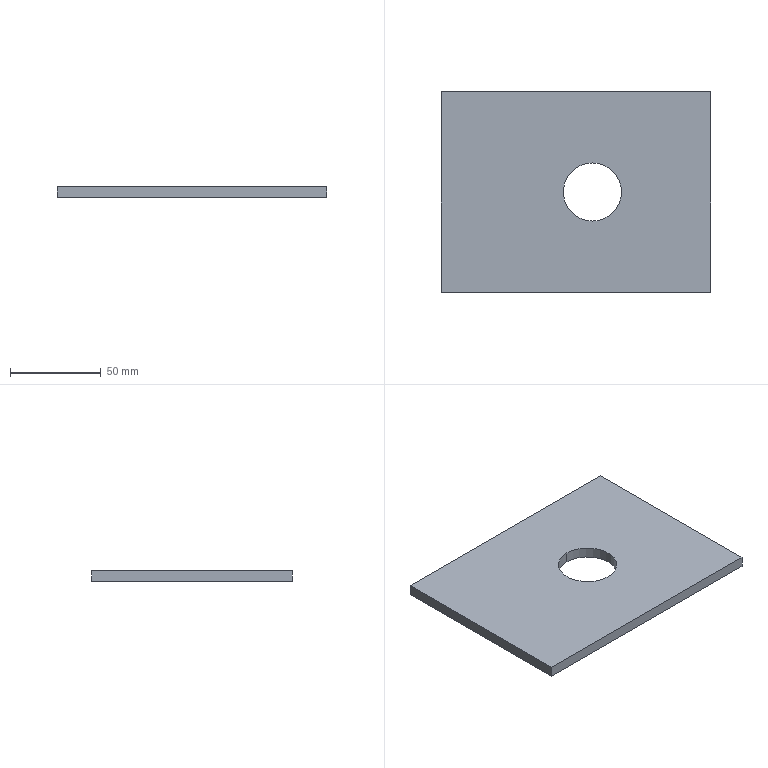Part | STEP file | 01-Pad plate | 1 solid | 8 faces | box 148 x 110 x 6 mm | volume 92855 mm3 | plane 6 | cylinder 2 | commonest cylinder face diameters 32 x2
STEP:
#1=CARTESIAN_POINT('',(0.,0.,0.));
#2=DIRECTION('',(0.,0.,1.));
#3=DIRECTION('',(1.,0.,0.));
#4=AXIS2_PLACEMENT_3D('',#1,#2,#3);
#5=CARTESIAN_POINT('',(83.,-39.,6.));
#6=VERTEX_POINT('',#5);
#7=CARTESIAN_POINT('',(83.,-39.,0.));
#8=VERTEX_POINT('',#7);
#9=CARTESIAN_POINT('',(83.,-39.,60.));
#10=DIRECTION('',(0.,0.,-1.));
#11=VECTOR('',#10,1.);
#12=LINE('',#9,#11);
#13=CARTESIAN_POINT('',(83.,-55.,60.));
#14=DIRECTION('',(0.,0.,-1.));
#15=DIRECTION('',(0.,1.,0.));
#16=AXIS2_PLACEMENT_3D('',#13,#14,#15);
#17=CYLINDRICAL_SURFACE('',#16,16.);
#18=CARTESIAN_POINT('',(6.283,0.));
#19=DIRECTION('',(0.,1.));
#20=VECTOR('',#19,1.);
#21=LINE('',#18,#20);
#22=(GEOMETRIC_REPRESENTATION_CONTEXT(2)PARAMETRIC_REPRESENTATION_CONTEXT()REPRESENTATION_CONTEXT('',''));
#23=DEFINITIONAL_REPRESENTATION('',(#21),#22);
#24=PCURVE('',#17,#23);
#25=CARTESIAN_POINT('',(83.,-55.,60.));
#26=DIRECTION('',(0.,0.,-1.));
#27=DIRECTION('',(0.,1.,0.));
#28=AXIS2_PLACEMENT_3D('',#25,#26,#27);
#29=CYLINDRICAL_SURFACE('',#28,16.);
#30=CARTESIAN_POINT('',(0.,0.));
#31=DIRECTION('',(0.,1.));
#32=VECTOR('',#31,1.);
#33=LINE('',#30,#32);
#34=(GEOMETRIC_REPRESENTATION_CONTEXT(2)PARAMETRIC_REPRESENTATION_CONTEXT()REPRESENTATION_CONTEXT('',''));
#35=DEFINITIONAL_REPRESENTATION('',(#33),#34);
#36=PCURVE('',#29,#35);
#37=SURFACE_CURVE('',#12,(#24,#36),.PCURVE_S1.);
#38=EDGE_CURVE('',#6,#8,#37,.T.);
#39=ORIENTED_EDGE('',*,*,#38,.T.);
#40=CARTESIAN_POINT('',(83.,-71.,0.));
#41=VERTEX_POINT('',#40);
#42=CARTESIAN_POINT('',(83.,-55.,0.));
#43=DIRECTION('',(0.,0.,-1.));
#44=DIRECTION('',(0.,1.,0.));
#45=AXIS2_PLACEMENT_3D('',#42,#43,#44);
#46=CIRCLE('',#45,16.);
#47=CARTESIAN_POINT('',(0.,60.));
#48=DIRECTION('',(1.,0.));
#49=VECTOR('',#48,1.);
#50=LINE('',#47,#49);
#51=(GEOMETRIC_REPRESENTATION_CONTEXT(2)PARAMETRIC_REPRESENTATION_CONTEXT()REPRESENTATION_CONTEXT('',''));
#52=DEFINITIONAL_REPRESENTATION('',(#50),#51);
#53=PCURVE('',#17,#52);
#54=CARTESIAN_POINT('',(0.,0.,0.));
#55=DIRECTION('',(0.,0.,1.));
#56=DIRECTION('',(1.,0.,0.));
#57=AXIS2_PLACEMENT_3D('',#54,#55,#56);
#58=PLANE('',#57);
#59=CARTESIAN_POINT('',(83.,-39.));
#60=CARTESIAN_POINT('',(110.713,-39.));
#61=CARTESIAN_POINT('',(96.856,-63.));
#62=CARTESIAN_POINT('',(83.,-87.));
#63=CARTESIAN_POINT('',(69.144,-63.));
#64=CARTESIAN_POINT('',(55.287,-39.));
#65=CARTESIAN_POINT('',(83.,-39.));
#66=(BOUNDED_CURVE()B_SPLINE_CURVE(2,(#59,#60,#61,#62,#63,#64,#65),.UNSPECIFIED.,.T.,.F.)B_SPLINE_CURVE_WITH_KNOTS((1,2,2,2,2,1),(-2.094,0.,2.094,4.189,6.283,8.378),.UNSPECIFIED.)CURVE()GEOMETRIC_REPRESENTATION_ITEM()RATIONAL_B_SPLINE_CURVE((1.,0.5,1.,0.5,1.,0.5,1.))REPRESENTATION_ITEM(''));
#67=(GEOMETRIC_REPRESENTATION_CONTEXT(2)PARAMETRIC_REPRESENTATION_CONTEXT()REPRESENTATION_CONTEXT('',''));
#68=DEFINITIONAL_REPRESENTATION('',(#66),#67);
#69=PCURVE('',#58,#68);
#70=SURFACE_CURVE('',#46,(#53,#69),.PCURVE_S1.);
#71=EDGE_CURVE('',#41,#8,#70,.T.);
#72=ORIENTED_EDGE('',*,*,#71,.F.);
#73=CARTESIAN_POINT('',(83.,-71.,6.));
#74=VERTEX_POINT('',#73);
#75=CARTESIAN_POINT('',(83.,-71.,60.));
#76=DIRECTION('',(0.,0.,-1.));
#77=VECTOR('',#76,1.);
#78=LINE('',#75,#77);
#79=CARTESIAN_POINT('',(3.142,0.));
#80=DIRECTION('',(0.,1.));
#81=VECTOR('',#80,1.);
#82=LINE('',#79,#81);
#83=(GEOMETRIC_REPRESENTATION_CONTEXT(2)PARAMETRIC_REPRESENTATION_CONTEXT()REPRESENTATION_CONTEXT('',''));
#84=DEFINITIONAL_REPRESENTATION('',(#82),#83);
#85=PCURVE('',#17,#84);
#86=CARTESIAN_POINT('',(3.142,0.));
#87=DIRECTION('',(0.,1.));
#88=VECTOR('',#87,1.);
#89=LINE('',#86,#88);
#90=(GEOMETRIC_REPRESENTATION_CONTEXT(2)PARAMETRIC_REPRESENTATION_CONTEXT()REPRESENTATION_CONTEXT('',''));
#91=DEFINITIONAL_REPRESENTATION('',(#89),#90);
#92=PCURVE('',#29,#91);
#93=SURFACE_CURVE('',#78,(#85,#92),.PCURVE_S1.);
#94=EDGE_CURVE('',#74,#41,#93,.T.);
#95=ORIENTED_EDGE('',*,*,#94,.F.);
#96=CARTESIAN_POINT('',(83.,-55.,6.));
#97=DIRECTION('',(0.,0.,1.));
#98=DIRECTION('',(0.,-1.,0.));
#99=AXIS2_PLACEMENT_3D('',#96,#97,#98);
#100=CIRCLE('',#99,16.);
#101=CARTESIAN_POINT('',(9.425,54.));
#102=DIRECTION('',(-1.,0.));
#103=VECTOR('',#102,1.);
#104=LINE('',#101,#103);
#105=(GEOMETRIC_REPRESENTATION_CONTEXT(2)PARAMETRIC_REPRESENTATION_CONTEXT()REPRESENTATION_CONTEXT('',''));
#106=DEFINITIONAL_REPRESENTATION('',(#104),#105);
#107=PCURVE('',#17,#106);
#108=CARTESIAN_POINT('',(0.,0.,6.));
#109=DIRECTION('',(0.,0.,1.));
#110=DIRECTION('',(1.,0.,0.));
#111=AXIS2_PLACEMENT_3D('',#108,#109,#110);
#112=PLANE('',#111);
#113=CARTESIAN_POINT('',(83.,-55.));
#114=DIRECTION('',(0.,-1.));
#115=AXIS2_PLACEMENT_2D('',#113,#114);
#116=CIRCLE('',#115,16.);
#117=(GEOMETRIC_REPRESENTATION_CONTEXT(2)PARAMETRIC_REPRESENTATION_CONTEXT()REPRESENTATION_CONTEXT('',''));
#118=DEFINITIONAL_REPRESENTATION('',(#116),#117);
#119=PCURVE('',#112,#118);
#120=SURFACE_CURVE('',#100,(#107,#119),.PCURVE_S1.);
#121=EDGE_CURVE('',#6,#74,#120,.T.);
#122=ORIENTED_EDGE('',*,*,#121,.F.);
#123=EDGE_LOOP('',(#39,#72,#95,#122));
#124=FACE_BOUND('',#123,.F.);
#125=ADVANCED_FACE('',(#124),#17,.F.);
#126=CARTESIAN_POINT('',(0.,0.,0.));
#127=VERTEX_POINT('',#126);
#128=CARTESIAN_POINT('',(0.,-110.,0.));
#129=VERTEX_POINT('',#128);
#130=CARTESIAN_POINT('',(0.,0.,0.));
#131=DIRECTION('',(0.,-1.,0.));
#132=VECTOR('',#131,1.);
#133=LINE('',#130,#132);
#134=CARTESIAN_POINT('',(0.,0.,6.));
#135=DIRECTION('',(1.,0.,0.));
#136=DIRECTION('',(0.,1.,0.));
#137=AXIS2_PLACEMENT_3D('',#134,#135,#136);
#138=PLANE('',#137);
#139=CARTESIAN_POINT('',(0.,-6.));
#140=DIRECTION('',(-1.,0.));
#141=VECTOR('',#140,1.);
#142=LINE('',#139,#141);
#143=(GEOMETRIC_REPRESENTATION_CONTEXT(2)PARAMETRIC_REPRESENTATION_CONTEXT()REPRESENTATION_CONTEXT('',''));
#144=DEFINITIONAL_REPRESENTATION('',(#142),#143);
#145=PCURVE('',#138,#144);
#146=CARTESIAN_POINT('',(0.,0.));
#147=DIRECTION('',(0.,-1.));
#148=VECTOR('',#147,1.);
#149=LINE('',#146,#148);
#150=(GEOMETRIC_REPRESENTATION_CONTEXT(2)PARAMETRIC_REPRESENTATION_CONTEXT()REPRESENTATION_CONTEXT('',''));
#151=DEFINITIONAL_REPRESENTATION('',(#149),#150);
#152=PCURVE('',#58,#151);
#153=SURFACE_CURVE('',#133,(#145,#152),.PCURVE_S1.);
#154=EDGE_CURVE('',#127,#129,#153,.T.);
#155=ORIENTED_EDGE('',*,*,#154,.T.);
#156=CARTESIAN_POINT('',(0.,-110.,6.));
#157=VERTEX_POINT('',#156);
#158=CARTESIAN_POINT('',(0.,-110.,6.));
#159=DIRECTION('',(0.,0.,-1.));
#160=VECTOR('',#159,1.);
#161=LINE('',#158,#160);
#162=CARTESIAN_POINT('',(-110.,0.));
#163=DIRECTION('',(0.,-1.));
#164=VECTOR('',#163,1.);
#165=LINE('',#162,#164);
#166=(GEOMETRIC_REPRESENTATION_CONTEXT(2)PARAMETRIC_REPRESENTATION_CONTEXT()REPRESENTATION_CONTEXT('',''));
#167=DEFINITIONAL_REPRESENTATION('',(#165),#166);
#168=PCURVE('',#138,#167);
#169=CARTESIAN_POINT('',(0.,-110.,6.));
#170=DIRECTION('',(0.,1.,0.));
#171=DIRECTION('',(0.,0.,1.));
#172=AXIS2_PLACEMENT_3D('',#169,#170,#171);
#173=PLANE('',#172);
#174=CARTESIAN_POINT('',(0.,0.));
#175=DIRECTION('',(-1.,0.));
#176=VECTOR('',#175,1.);
#177=LINE('',#174,#176);
#178=(GEOMETRIC_REPRESENTATION_CONTEXT(2)PARAMETRIC_REPRESENTATION_CONTEXT()REPRESENTATION_CONTEXT('',''));
#179=DEFINITIONAL_REPRESENTATION('',(#177),#178);
#180=PCURVE('',#173,#179);
#181=SURFACE_CURVE('',#161,(#168,#180),.PCURVE_S1.);
#182=EDGE_CURVE('',#157,#129,#181,.T.);
#183=ORIENTED_EDGE('',*,*,#182,.F.);
#184=CARTESIAN_POINT('',(0.,0.,6.));
#185=VERTEX_POINT('',#184);
#186=CARTESIAN_POINT('',(0.,0.,6.));
#187=DIRECTION('',(0.,-1.,0.));
#188=VECTOR('',#187,1.);
#189=LINE('',#186,#188);
#190=CARTESIAN_POINT('',(0.,0.));
#191=DIRECTION('',(-1.,0.));
#192=VECTOR('',#191,1.);
#193=LINE('',#190,#192);
#194=(GEOMETRIC_REPRESENTATION_CONTEXT(2)PARAMETRIC_REPRESENTATION_CONTEXT()REPRESENTATION_CONTEXT('',''));
#195=DEFINITIONAL_REPRESENTATION('',(#193),#194);
#196=PCURVE('',#138,#195);
#197=CARTESIAN_POINT('',(0.,0.));
#198=DIRECTION('',(0.,-1.));
#199=VECTOR('',#198,1.);
#200=LINE('',#197,#199);
#201=(GEOMETRIC_REPRESENTATION_CONTEXT(2)PARAMETRIC_REPRESENTATION_CONTEXT()REPRESENTATION_CONTEXT('',''));
#202=DEFINITIONAL_REPRESENTATION('',(#200),#201);
#203=PCURVE('',#112,#202);
#204=SURFACE_CURVE('',#189,(#196,#203),.PCURVE_S1.);
#205=EDGE_CURVE('',#185,#157,#204,.T.);
#206=ORIENTED_EDGE('',*,*,#205,.F.);
#207=CARTESIAN_POINT('',(0.,0.,6.));
#208=DIRECTION('',(0.,0.,-1.));
#209=VECTOR('',#208,1.);
#210=LINE('',#207,#209);
#211=CARTESIAN_POINT('',(0.,0.));
#212=DIRECTION('',(0.,-1.));
#213=VECTOR('',#212,1.);
#214=LINE('',#211,#213);
#215=(GEOMETRIC_REPRESENTATION_CONTEXT(2)PARAMETRIC_REPRESENTATION_CONTEXT()REPRESENTATION_CONTEXT('',''));
#216=DEFINITIONAL_REPRESENTATION('',(#214),#215);
#217=PCURVE('',#138,#216);
#218=CARTESIAN_POINT('',(0.,0.,6.));
#219=DIRECTION('',(0.,-1.,0.));
#220=DIRECTION('',(0.,0.,-1.));
#221=AXIS2_PLACEMENT_3D('',#218,#219,#220);
#222=PLANE('',#221);
#223=CARTESIAN_POINT('',(0.,0.));
#224=DIRECTION('',(1.,0.));
#225=VECTOR('',#224,1.);
#226=LINE('',#223,#225);
#227=(GEOMETRIC_REPRESENTATION_CONTEXT(2)PARAMETRIC_REPRESENTATION_CONTEXT()REPRESENTATION_CONTEXT('',''));
#228=DEFINITIONAL_REPRESENTATION('',(#226),#227);
#229=PCURVE('',#222,#228);
#230=SURFACE_CURVE('',#210,(#217,#229),.PCURVE_S1.);
#231=EDGE_CURVE('',#185,#127,#230,.T.);
#232=ORIENTED_EDGE('',*,*,#231,.T.);
#233=EDGE_LOOP('',(#155,#183,#206,#232));
#234=FACE_BOUND('',#233,.T.);
#235=ADVANCED_FACE('',(#234),#138,.F.);
#236=CARTESIAN_POINT('',(148.,-110.,0.));
#237=VERTEX_POINT('',#236);
#238=CARTESIAN_POINT('',(0.,-110.,0.));
#239=DIRECTION('',(1.,0.,0.));
#240=VECTOR('',#239,1.);
#241=LINE('',#238,#240);
#242=CARTESIAN_POINT('',(-6.,0.));
#243=DIRECTION('',(0.,1.));
#244=VECTOR('',#243,1.);
#245=LINE('',#242,#244);
#246=(GEOMETRIC_REPRESENTATION_CONTEXT(2)PARAMETRIC_REPRESENTATION_CONTEXT()REPRESENTATION_CONTEXT('',''));
#247=DEFINITIONAL_REPRESENTATION('',(#245),#246);
#248=PCURVE('',#173,#247);
#249=CARTESIAN_POINT('',(0.,-110.));
#250=DIRECTION('',(1.,0.));
#251=VECTOR('',#250,1.);
#252=LINE('',#249,#251);
#253=(GEOMETRIC_REPRESENTATION_CONTEXT(2)PARAMETRIC_REPRESENTATION_CONTEXT()REPRESENTATION_CONTEXT('',''));
#254=DEFINITIONAL_REPRESENTATION('',(#252),#253);
#255=PCURVE('',#58,#254);
#256=SURFACE_CURVE('',#241,(#248,#255),.PCURVE_S1.);
#257=EDGE_CURVE('',#129,#237,#256,.T.);
#258=ORIENTED_EDGE('',*,*,#257,.T.);
#259=CARTESIAN_POINT('',(148.,-110.,6.));
#260=VERTEX_POINT('',#259);
#261=CARTESIAN_POINT('',(148.,-110.,6.));
#262=DIRECTION('',(0.,0.,-1.));
#263=VECTOR('',#262,1.);
#264=LINE('',#261,#263);
#265=CARTESIAN_POINT('',(0.,148.));
#266=DIRECTION('',(-1.,0.));
#267=VECTOR('',#266,1.);
#268=LINE('',#265,#267);
#269=(GEOMETRIC_REPRESENTATION_CONTEXT(2)PARAMETRIC_REPRESENTATION_CONTEXT()REPRESENTATION_CONTEXT('',''));
#270=DEFINITIONAL_REPRESENTATION('',(#268),#269);
#271=PCURVE('',#173,#270);
#272=CARTESIAN_POINT('',(148.,0.,6.));
#273=DIRECTION('',(-1.,0.,0.));
#274=DIRECTION('',(0.,0.,1.));
#275=AXIS2_PLACEMENT_3D('',#272,#273,#274);
#276=PLANE('',#275);
#277=CARTESIAN_POINT('',(0.,-110.));
#278=DIRECTION('',(-1.,0.));
#279=VECTOR('',#278,1.);
#280=LINE('',#277,#279);
#281=(GEOMETRIC_REPRESENTATION_CONTEXT(2)PARAMETRIC_REPRESENTATION_CONTEXT()REPRESENTATION_CONTEXT('',''));
#282=DEFINITIONAL_REPRESENTATION('',(#280),#281);
#283=PCURVE('',#276,#282);
#284=SURFACE_CURVE('',#264,(#271,#283),.PCURVE_S1.);
#285=EDGE_CURVE('',#260,#237,#284,.T.);
#286=ORIENTED_EDGE('',*,*,#285,.F.);
#287=CARTESIAN_POINT('',(0.,-110.,6.));
#288=DIRECTION('',(1.,0.,0.));
#289=VECTOR('',#288,1.);
#290=LINE('',#287,#289);
#291=CARTESIAN_POINT('',(0.,0.));
#292=DIRECTION('',(0.,1.));
#293=VECTOR('',#292,1.);
#294=LINE('',#291,#293);
#295=(GEOMETRIC_REPRESENTATION_CONTEXT(2)PARAMETRIC_REPRESENTATION_CONTEXT()REPRESENTATION_CONTEXT('',''));
#296=DEFINITIONAL_REPRESENTATION('',(#294),#295);
#297=PCURVE('',#173,#296);
#298=CARTESIAN_POINT('',(0.,-110.));
#299=DIRECTION('',(1.,0.));
#300=VECTOR('',#299,1.);
#301=LINE('',#298,#300);
#302=(GEOMETRIC_REPRESENTATION_CONTEXT(2)PARAMETRIC_REPRESENTATION_CONTEXT()REPRESENTATION_CONTEXT('',''));
#303=DEFINITIONAL_REPRESENTATION('',(#301),#302);
#304=PCURVE('',#112,#303);
#305=SURFACE_CURVE('',#290,(#297,#304),.PCURVE_S1.);
#306=EDGE_CURVE('',#157,#260,#305,.T.);
#307=ORIENTED_EDGE('',*,*,#306,.F.);
#308=ORIENTED_EDGE('',*,*,#182,.T.);
#309=EDGE_LOOP('',(#258,#286,#307,#308));
#310=FACE_BOUND('',#309,.T.);
#311=ADVANCED_FACE('',(#310),#173,.F.);
#312=CARTESIAN_POINT('',(148.,0.,0.));
#313=VERTEX_POINT('',#312);
#314=CARTESIAN_POINT('',(148.,0.,0.));
#315=DIRECTION('',(0.,1.,0.));
#316=VECTOR('',#315,1.);
#317=LINE('',#314,#316);
#318=CARTESIAN_POINT('',(-6.,0.));
#319=DIRECTION('',(0.,1.));
#320=VECTOR('',#319,1.);
#321=LINE('',#318,#320);
#322=(GEOMETRIC_REPRESENTATION_CONTEXT(2)PARAMETRIC_REPRESENTATION_CONTEXT()REPRESENTATION_CONTEXT('',''));
#323=DEFINITIONAL_REPRESENTATION('',(#321),#322);
#324=PCURVE('',#276,#323);
#325=CARTESIAN_POINT('',(148.,0.));
#326=DIRECTION('',(0.,1.));
#327=VECTOR('',#326,1.);
#328=LINE('',#325,#327);
#329=(GEOMETRIC_REPRESENTATION_CONTEXT(2)PARAMETRIC_REPRESENTATION_CONTEXT()REPRESENTATION_CONTEXT('',''));
#330=DEFINITIONAL_REPRESENTATION('',(#328),#329);
#331=PCURVE('',#58,#330);
#332=SURFACE_CURVE('',#317,(#324,#331),.PCURVE_S1.);
#333=EDGE_CURVE('',#237,#313,#332,.T.);
#334=ORIENTED_EDGE('',*,*,#333,.T.);
#335=CARTESIAN_POINT('',(148.,0.,6.));
#336=VERTEX_POINT('',#335);
#337=CARTESIAN_POINT('',(148.,0.,6.));
#338=DIRECTION('',(0.,0.,-1.));
#339=VECTOR('',#338,1.);
#340=LINE('',#337,#339);
#341=CARTESIAN_POINT('',(0.,0.));
#342=DIRECTION('',(-1.,0.));
#343=VECTOR('',#342,1.);
#344=LINE('',#341,#343);
#345=(GEOMETRIC_REPRESENTATION_CONTEXT(2)PARAMETRIC_REPRESENTATION_CONTEXT()REPRESENTATION_CONTEXT('',''));
#346=DEFINITIONAL_REPRESENTATION('',(#344),#345);
#347=PCURVE('',#276,#346);
#348=CARTESIAN_POINT('',(0.,148.));
#349=DIRECTION('',(1.,0.));
#350=VECTOR('',#349,1.);
#351=LINE('',#348,#350);
#352=(GEOMETRIC_REPRESENTATION_CONTEXT(2)PARAMETRIC_REPRESENTATION_CONTEXT()REPRESENTATION_CONTEXT('',''));
#353=DEFINITIONAL_REPRESENTATION('',(#351),#352);
#354=PCURVE('',#222,#353);
#355=SURFACE_CURVE('',#340,(#347,#354),.PCURVE_S1.);
#356=EDGE_CURVE('',#336,#313,#355,.T.);
#357=ORIENTED_EDGE('',*,*,#356,.F.);
#358=CARTESIAN_POINT('',(148.,0.,6.));
#359=DIRECTION('',(0.,1.,0.));
#360=VECTOR('',#359,1.);
#361=LINE('',#358,#360);
#362=CARTESIAN_POINT('',(0.,0.));
#363=DIRECTION('',(0.,1.));
#364=VECTOR('',#363,1.);
#365=LINE('',#362,#364);
#366=(GEOMETRIC_REPRESENTATION_CONTEXT(2)PARAMETRIC_REPRESENTATION_CONTEXT()REPRESENTATION_CONTEXT('',''));
#367=DEFINITIONAL_REPRESENTATION('',(#365),#366);
#368=PCURVE('',#276,#367);
#369=CARTESIAN_POINT('',(148.,0.));
#370=DIRECTION('',(0.,1.));
#371=VECTOR('',#370,1.);
#372=LINE('',#369,#371);
#373=(GEOMETRIC_REPRESENTATION_CONTEXT(2)PARAMETRIC_REPRESENTATION_CONTEXT()REPRESENTATION_CONTEXT('',''));
#374=DEFINITIONAL_REPRESENTATION('',(#372),#373);
#375=PCURVE('',#112,#374);
#376=SURFACE_CURVE('',#361,(#368,#375),.PCURVE_S1.);
#377=EDGE_CURVE('',#260,#336,#376,.T.);
#378=ORIENTED_EDGE('',*,*,#377,.F.);
#379=ORIENTED_EDGE('',*,*,#285,.T.);
#380=EDGE_LOOP('',(#334,#357,#378,#379));
#381=FACE_BOUND('',#380,.T.);
#382=ADVANCED_FACE('',(#381),#276,.F.);
#383=CARTESIAN_POINT('',(0.,0.,0.));
#384=DIRECTION('',(-1.,0.,0.));
#385=VECTOR('',#384,1.);
#386=LINE('',#383,#385);
#387=CARTESIAN_POINT('',(6.,0.));
#388=DIRECTION('',(0.,-1.));
#389=VECTOR('',#388,1.);
#390=LINE('',#387,#389);
#391=(GEOMETRIC_REPRESENTATION_CONTEXT(2)PARAMETRIC_REPRESENTATION_CONTEXT()REPRESENTATION_CONTEXT('',''));
#392=DEFINITIONAL_REPRESENTATION('',(#390),#391);
#393=PCURVE('',#222,#392);
#394=CARTESIAN_POINT('',(0.,0.));
#395=DIRECTION('',(-1.,0.));
#396=VECTOR('',#395,1.);
#397=LINE('',#394,#396);
#398=(GEOMETRIC_REPRESENTATION_CONTEXT(2)PARAMETRIC_REPRESENTATION_CONTEXT()REPRESENTATION_CONTEXT('',''));
#399=DEFINITIONAL_REPRESENTATION('',(#397),#398);
#400=PCURVE('',#58,#399);
#401=SURFACE_CURVE('',#386,(#393,#400),.PCURVE_S1.);
#402=EDGE_CURVE('',#313,#127,#401,.T.);
#403=ORIENTED_EDGE('',*,*,#402,.T.);
#404=ORIENTED_EDGE('',*,*,#231,.F.);
#405=CARTESIAN_POINT('',(0.,0.,6.));
#406=DIRECTION('',(-1.,0.,0.));
#407=VECTOR('',#406,1.);
#408=LINE('',#405,#407);
#409=CARTESIAN_POINT('',(0.,0.));
#410=DIRECTION('',(0.,-1.));
#411=VECTOR('',#410,1.);
#412=LINE('',#409,#411);
#413=(GEOMETRIC_REPRESENTATION_CONTEXT(2)PARAMETRIC_REPRESENTATION_CONTEXT()REPRESENTATION_CONTEXT('',''));
#414=DEFINITIONAL_REPRESENTATION('',(#412),#413);
#415=PCURVE('',#222,#414);
#416=CARTESIAN_POINT('',(0.,0.));
#417=DIRECTION('',(-1.,0.));
#418=VECTOR('',#417,1.);
#419=LINE('',#416,#418);
#420=(GEOMETRIC_REPRESENTATION_CONTEXT(2)PARAMETRIC_REPRESENTATION_CONTEXT()REPRESENTATION_CONTEXT('',''));
#421=DEFINITIONAL_REPRESENTATION('',(#419),#420);
#422=PCURVE('',#112,#421);
#423=SURFACE_CURVE('',#408,(#415,#422),.PCURVE_S1.);
#424=EDGE_CURVE('',#336,#185,#423,.T.);
#425=ORIENTED_EDGE('',*,*,#424,.F.);
#426=ORIENTED_EDGE('',*,*,#356,.T.);
#427=EDGE_LOOP('',(#403,#404,#425,#426));
#428=FACE_BOUND('',#427,.T.);
#429=ADVANCED_FACE('',(#428),#222,.F.);
#430=ORIENTED_EDGE('',*,*,#121,.F.);
#431=CARTESIAN_POINT('',(83.,-55.,6.));
#432=DIRECTION('',(0.,0.,1.));
#433=DIRECTION('',(0.,-1.,0.));
#434=AXIS2_PLACEMENT_3D('',#431,#432,#433);
#435=CIRCLE('',#434,16.);
#436=CARTESIAN_POINT('',(83.,-55.));
#437=DIRECTION('',(0.,-1.));
#438=AXIS2_PLACEMENT_2D('',#436,#437);
#439=CIRCLE('',#438,16.);
#440=(GEOMETRIC_REPRESENTATION_CONTEXT(2)PARAMETRIC_REPRESENTATION_CONTEXT()REPRESENTATION_CONTEXT('',''));
#441=DEFINITIONAL_REPRESENTATION('',(#439),#440);
#442=PCURVE('',#112,#441);
#443=CARTESIAN_POINT('',(3.142,54.));
#444=DIRECTION('',(-1.,0.));
#445=VECTOR('',#444,1.);
#446=LINE('',#443,#445);
#447=(GEOMETRIC_REPRESENTATION_CONTEXT(2)PARAMETRIC_REPRESENTATION_CONTEXT()REPRESENTATION_CONTEXT('',''));
#448=DEFINITIONAL_REPRESENTATION('',(#446),#447);
#449=PCURVE('',#29,#448);
#450=SURFACE_CURVE('',#435,(#442,#449),.PCURVE_S1.);
#451=EDGE_CURVE('',#74,#6,#450,.T.);
#452=ORIENTED_EDGE('',*,*,#451,.F.);
#453=EDGE_LOOP('',(#430,#452));
#454=FACE_BOUND('',#453,.T.);
#455=ORIENTED_EDGE('',*,*,#205,.T.);
#456=ORIENTED_EDGE('',*,*,#306,.T.);
#457=ORIENTED_EDGE('',*,*,#377,.T.);
#458=ORIENTED_EDGE('',*,*,#424,.T.);
#459=EDGE_LOOP('',(#455,#456,#457,#458));
#460=FACE_BOUND('',#459,.T.);
#461=ADVANCED_FACE('',(#454,#460),#112,.T.);
#462=CARTESIAN_POINT('',(83.,-55.,0.));
#463=DIRECTION('',(0.,0.,-1.));
#464=DIRECTION('',(0.,1.,0.));
#465=AXIS2_PLACEMENT_3D('',#462,#463,#464);
#466=CIRCLE('',#465,16.);
#467=CARTESIAN_POINT('',(83.,-39.));
#468=CARTESIAN_POINT('',(110.713,-39.));
#469=CARTESIAN_POINT('',(96.856,-63.));
#470=CARTESIAN_POINT('',(83.,-87.));
#471=CARTESIAN_POINT('',(69.144,-63.));
#472=CARTESIAN_POINT('',(55.287,-39.));
#473=CARTESIAN_POINT('',(83.,-39.));
#474=(BOUNDED_CURVE()B_SPLINE_CURVE(2,(#467,#468,#469,#470,#471,#472,#473),.UNSPECIFIED.,.T.,.F.)B_SPLINE_CURVE_WITH_KNOTS((1,2,2,2,2,1),(-2.094,0.,2.094,4.189,6.283,8.378),.UNSPECIFIED.)CURVE()GEOMETRIC_REPRESENTATION_ITEM()RATIONAL_B_SPLINE_CURVE((1.,0.5,1.,0.5,1.,0.5,1.))REPRESENTATION_ITEM(''));
#475=(GEOMETRIC_REPRESENTATION_CONTEXT(2)PARAMETRIC_REPRESENTATION_CONTEXT()REPRESENTATION_CONTEXT('',''));
#476=DEFINITIONAL_REPRESENTATION('',(#474),#475);
#477=PCURVE('',#58,#476);
#478=CARTESIAN_POINT('',(0.,60.));
#479=DIRECTION('',(1.,0.));
#480=VECTOR('',#479,1.);
#481=LINE('',#478,#480);
#482=(GEOMETRIC_REPRESENTATION_CONTEXT(2)PARAMETRIC_REPRESENTATION_CONTEXT()REPRESENTATION_CONTEXT('',''));
#483=DEFINITIONAL_REPRESENTATION('',(#481),#482);
#484=PCURVE('',#29,#483);
#485=SURFACE_CURVE('',#466,(#477,#484),.PCURVE_S1.);
#486=EDGE_CURVE('',#8,#41,#485,.T.);
#487=ORIENTED_EDGE('',*,*,#486,.F.);
#488=ORIENTED_EDGE('',*,*,#71,.F.);
#489=EDGE_LOOP('',(#487,#488));
#490=FACE_BOUND('',#489,.T.);
#491=ORIENTED_EDGE('',*,*,#154,.F.);
#492=ORIENTED_EDGE('',*,*,#402,.F.);
#493=ORIENTED_EDGE('',*,*,#333,.F.);
#494=ORIENTED_EDGE('',*,*,#257,.F.);
#495=EDGE_LOOP('',(#491,#492,#493,#494));
#496=FACE_BOUND('',#495,.T.);
#497=ADVANCED_FACE('',(#490,#496),#58,.F.);
#498=ORIENTED_EDGE('',*,*,#486,.F.);
#499=ORIENTED_EDGE('',*,*,#38,.F.);
#500=ORIENTED_EDGE('',*,*,#451,.F.);
#501=ORIENTED_EDGE('',*,*,#94,.T.);
#502=EDGE_LOOP('',(#498,#499,#500,#501));
#503=FACE_BOUND('',#502,.F.);
#504=ADVANCED_FACE('',(#503),#29,.F.);
#505=CLOSED_SHELL('',(#125,#235,#311,#382,#429,#461,#497,#504));
#506=MANIFOLD_SOLID_BREP('',#505);
#507=(LENGTH_UNIT()NAMED_UNIT(*)SI_UNIT(.MILLI.,.METRE.));
#508=UNCERTAINTY_MEASURE_WITH_UNIT(LENGTH_MEASURE(0.0000001),#507,'','');
#509=(NAMED_UNIT(*)PLANE_ANGLE_UNIT()SI_UNIT($,.RADIAN.));
#510=(NAMED_UNIT(*)SI_UNIT($,.STERADIAN.)SOLID_ANGLE_UNIT());
#511=(GEOMETRIC_REPRESENTATION_CONTEXT(3)GLOBAL_UNCERTAINTY_ASSIGNED_CONTEXT((#508))GLOBAL_UNIT_ASSIGNED_CONTEXT((#507,#509,#510))REPRESENTATION_CONTEXT('',''));
#512=ADVANCED_BREP_SHAPE_REPRESENTATION('',(#4,#506),#511);